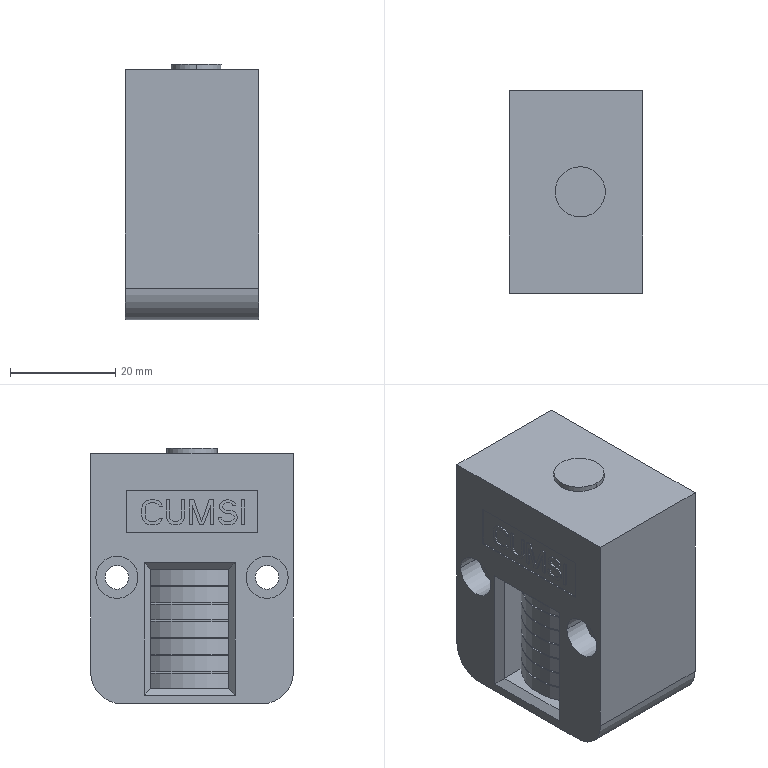Part | Creo | 1 solid | 201 faces | box 25.4 x 38.5 x 48.5 mm | volume 43523 mm3 | plane 182 | cylinder 19 | commonest cylinder face diameters 22 x7 4.5 x4 8 x4 9.525 x2 12 x2